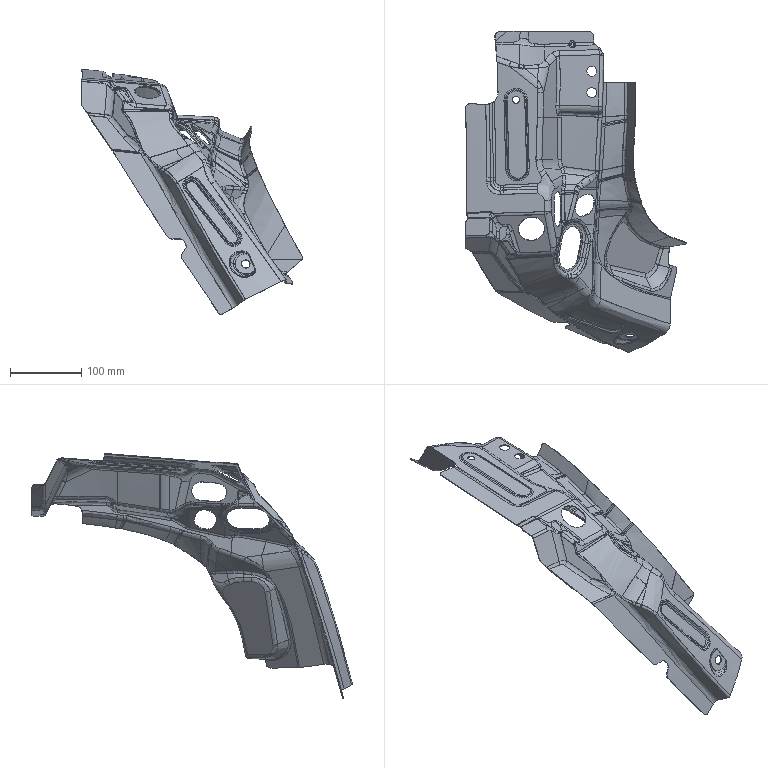Part | STEP file | FNA5401771 | 1 solid | 957 faces | box 311.119 x 450.581 x 343.825 mm | volume 154298 mm3 | spline 794 | cylinder 90 | plane 46 | other 23 | sphere 4 | commonest cylinder face diameters 12 x15 10 x12 14 x11 18 x11 16 x9 20 x6